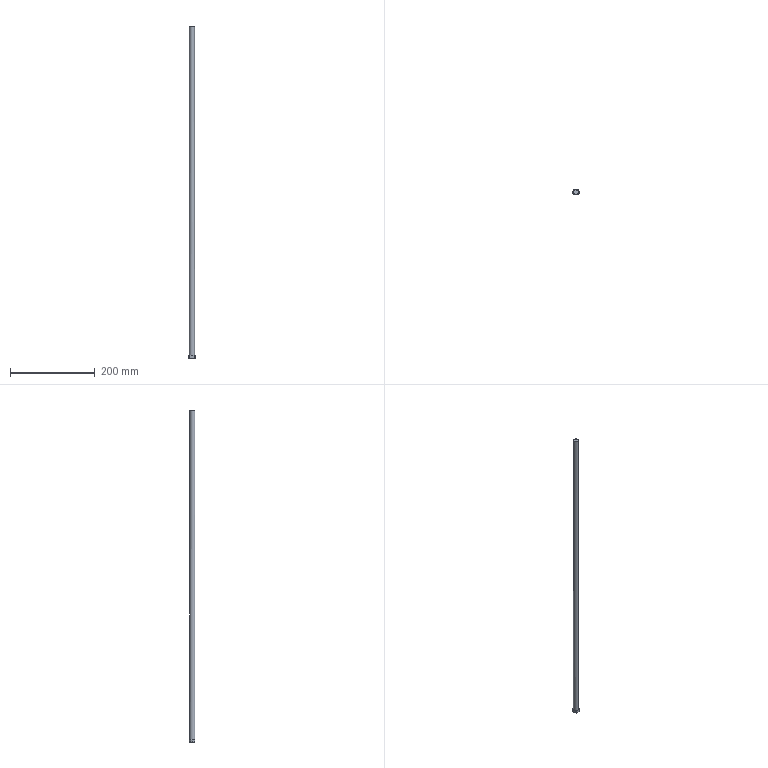Part | STEP file | solid 60 | 1 solid | 45 faces | box 16 x 14 x 783.319 mm | volume 88933 mm3 | plane 24 | other 15 | cylinder 2 | cone 2 | torus 1 | spline 1 | commonest cylinder face diameters 12 x1 16 x1